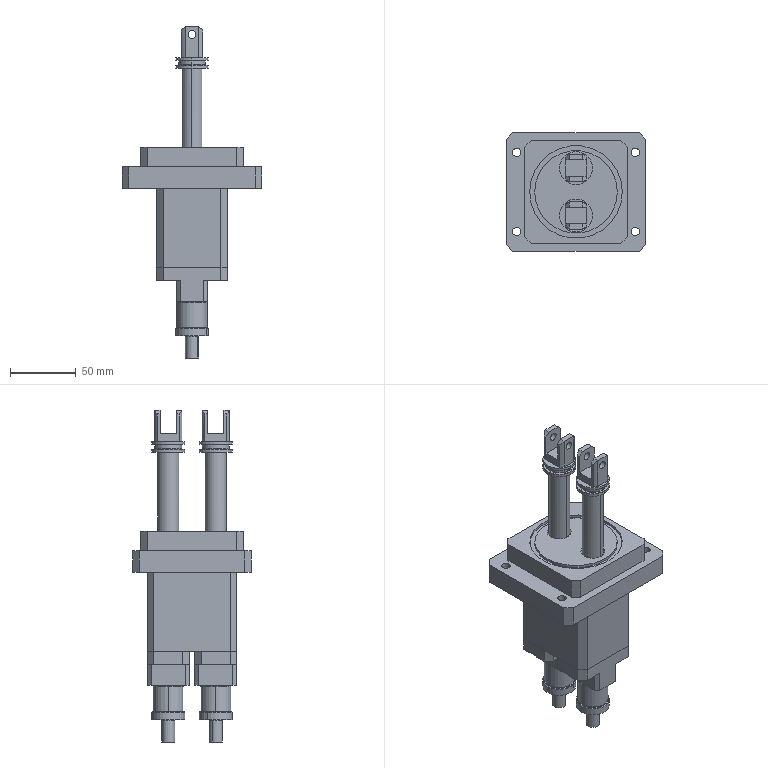Part | SolidWorks | 9 solids | 380 faces | box 106 x 90 x 252 mm | volume 546478 mm3 | plane 144 | cylinder 140 | cone 64 | torus 32 | commonest cylinder face diameters 10 x16 16 x12 23 x12 25 x12 4.2 x8 5 x8